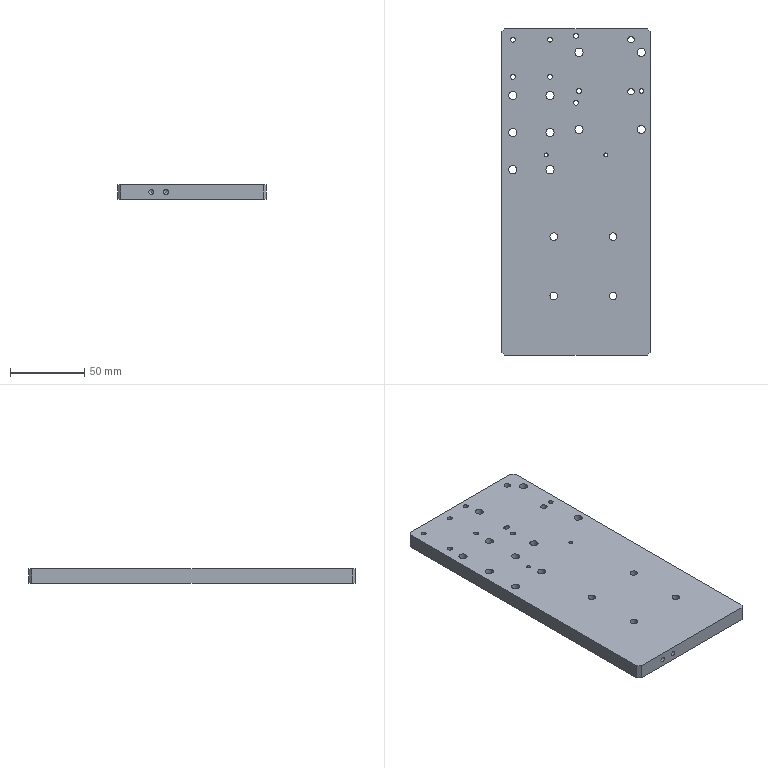CAM job | NX | 3-axis milling, drilling | part box 100 x 220 x 10 mm | stock box 105 x 225 x 12 mm
Tools:
number,name,description,diameter,corner_radius,flute_length,length,flutes
19,D2,平底铣刀-粗,2.0,0.0,50.0,75.0,2
4,D4,平底铣刀-粗,4.0,0.0,25.0,75.0,2
6,D6,平底铣刀-粗,6.0,0.0,25.0,75.0,2
9,D10,平底铣刀-粗,10.0,0.0,35.0,75.0,2
23,D2-J,平底铣刀-精,2.0,0.0,50.0,75.0,2
11,D4-J,平底铣刀-精,4.0,0.0,50.0,75.0,2
7,D6-J,平底铣刀-精,6.0,0.0,25.0,75.0,2
10,D10-J,平底铣刀-精,10.0,0.0,35.0,75.0,2
1,D80R0.8飞刀,圆鼻刀-粗,80.0,0.8,50.0,75.0,2
1,D80R0.8飞刀-J,圆鼻刀-精,80.0,0.8,50.0,75.0,2
2,D6倒角刀,倒角刀,6.0,0.0,3.0,25.0,2
20,M3X0.5,丝锥,2.5,0.0,35.0,50.0,2
21,M4X0.7,丝锥,3.3,0.0,35.0,50.0,2
22,M5X0.8,丝锥,4.2,0.0,35.0,50.0,2
16,M6X1.0,丝锥,5.0,0.0,35.0,50.0,2
24,D3铰刀,Drilling Tool,3.0,0.0,75.0,100.0,6
12,ZT2.5,钻头,2.5,0.0,35.0,50.0,2
15,ZT5,钻头,5.0,0.0,35.0,50.0,2
18,ZT5.5,钻头,5.5,0.0,35.0,50.0,2
13,钻头3.3,Twist Drill 3.3 mm,3.3,0.0,35.0,35.008,2
14,钻头4.2,Twist Drill 4.2 mm,4.2,0.0,41.0,41.738,2
17,ZT2.9,Drilling Tool,2.9,0.0,35.0,50.0,2
Operations:
program,operation,operation_type,tool,method,geometry_group,spindle_rpm,surface_speed,feed_per_tooth,feed_cut,feed_plunge,cut_length_mm,path_length_mm,cut_time_min,machine_time_min
B,底壁铣飞面开粗_COPY,VolumeBased25DMillingOperation,D80R0.8飞刀,分层开粗-切深K-步距G,W-B,2800.0,703.696,0.5357,3000.0,100.0,2666.79,2835.673,0.8889,0.9058
B,底壁铣飞面精光_COPY,VolumeBased25DMillingOperation,D80R0.8飞刀-J,侧刃精光-切深K-步距G,W-B,4000.0,1005.28,0.125,1000.0,100.0,666.11,702.11,0.6661,0.6697
B,钻倒角_4,Operation,D6倒角刀,METHOD,W-B,8000.0,150.796,0.0625,1000.0,0.0,9.5,102.112,0.0095,0.0188
B,钻倒角_5,Operation,D6倒角刀,METHOD,W-B,8000.0,150.796,0.0625,1000.0,0.0,4.8,49.6,0.0048,0.0093
B,钻倒角_6,Operation,D6倒角刀,METHOD,W-B,8000.0,150.796,0.0625,1000.0,0.0,31.2,235.798,0.0312,0.0517
B,钻倒角_7,Operation,D6倒角刀,METHOD,W-B,8000.0,150.796,0.0625,1000.0,0.0,11.4,100.928,0.0114,0.0204
B,铣倒角_5,PlanarMilling,D6倒角刀,METHOD,W-B,8000.0,150.796,0.0375,600.0,100.0,75.821,364.836,0.1264,0.1553
B,铣倒角_6,PlanarMilling,D6倒角刀,METHOD,W-B,8000.0,150.796,0.075,1200.0,100.0,177.946,861.886,0.1483,0.2167
B,C0.3封闭铣廓倒角6X45L_COPY,PlanarMilling,D6倒角刀,爬面_倒角-切深0-步距G,W-B,7000.0,131.0,0.1071,1500.0,100.0,673.102,930.341,0.4487,0.4745
A,顶面,FaceMilling,D80R0.8飞刀,侧刃精光-切深K-步距G,W-A,4000.0,1005.31,0.125,1000.0,100.0,1004.0,1040.0,1.004,1.008
A,外形粗_2,VolumeBased25DMillingOperation,D10,METHOD,W-A,8000.0,251.327,0.3125,5000.0,80.0,10011.875,10060.475,2.002,2.007
A,打点-深0.8,Operation,D6倒角刀,NONE,W-A,8000.0,150.796,0.0312,500.0,90.0,50.4,871.238,0.1008,0.1829
A,通孔-M3螺纹底孔,Operation,ZT2.5,NONE,W-A,3000.0,23.562,0.05,300.0,90.0,33.502,148.017,0.1117,0.1231
A,通孔-精孔3.0预钻,Operation,ZT2.9,NONE,W-A,3200.0,29.154,0.0312,200.0,90.0,29.674,141.861,0.1484,0.1596
A,通孔-M4螺纹底孔,Operation,钻头3.3,NONE,W-A,3000.0,31.102,0.05,300.0,90.0,101.948,366.432,0.3398,0.3663
A,通孔-M5螺纹底孔,Operation,钻头4.2,NONE,W-A,3000.0,39.584,0.0583,350.0,90.0,36.524,149.061,0.1044,0.1156
A,通孔-M6螺纹底孔,Operation,ZT5,NONE,W-A,2800.0,43.982,0.0625,350.0,90.0,74.009,311.055,0.2115,0.2352
A,沉头孔-钻孔0段,Operation,ZT5.5,NONE,W-A,1200.0,20.735,0.0625,150.0,90.0,146.524,605.76,0.9768,1.023
A,通孔-精孔6.0预钻14.8,Operation,ZT5.5,NONE,W-A,2500.0,45.553,0.03,150.0,90.0,19.405,119.823,0.1294,0.1394
A,通腰槽粗_1,VolumeBased25DMillingOperation,D2,METHOD,W-A,6000.0,37.699,0.0417,500.0,100.0,522.974,571.674,1.046,1.051
A,铣孔开粗D6_1,CylinderMilling,D6,NONE,W-A,8000.0,150.796,0.075,1200.0,100.0,1588.996,2301.545,1.324,1.395
A,铣孔开粗D4_1,CylinderMilling,D4,NONE,W-A,8000.0,100.531,0.0375,600.0,100.0,313.409,446.409,0.5223,0.5356
A,铣孔精光D6_1,CylinderMilling,D6-J,精光步距切深关,W-A,8000.0,150.796,0.0312,500.0,100.0,333.986,1051.534,0.668,0.7397
A,仅选体,SurfaceContour,D6倒角刀,METHOD,W-A,8000.0,150.796,0.1875,3000.0,100.0,665.713,820.009,0.2219,0.2373
A,钻倒角_1,Operation,D6倒角刀,METHOD,W-A,8000.0,150.796,0.0312,500.0,0.0,9.5,102.112,0.019,0.0283
A,钻倒角_2,Operation,D6倒角刀,METHOD,W-A,8000.0,150.796,0.0312,500.0,0.0,4.8,49.6,0.0096,0.0141
A,钻倒角_3,Operation,D6倒角刀,METHOD,W-A,8000.0,150.796,0.0312,500.0,0.0,31.2,235.798,0.0624,0.0829
A,铣倒角_1,PlanarMilling,D6倒角刀,METHOD,W-A,8000.0,150.796,0.0312,500.0,100.0,36.041,154.428,0.0721,0.0839
A,铣倒角_2,PlanarMilling,D6倒角刀,METHOD,W-A,8000.0,150.796,0.0312,500.0,100.0,79.753,364.605,0.1595,0.188
A,铣倒角_3,PlanarMilling,D6倒角刀,METHOD,W-A,8000.0,150.796,0.0312,500.0,100.0,41.927,161.633,0.0839,0.0958
A,铣倒角_4,PlanarMilling,D6倒角刀,NONE,W-A,8000.0,150.796,0.05,800.0,100.0,402.51,1022.014,0.5031,0.5651
A,铣孔精光D4-J_1,CylinderMilling,D4-J,精光步距切深关,W-A,8000.0,100.531,0.0125,200.0,100.0,115.195,248.195,0.576,0.5893
A,腰槽精_1,VolumeBased25DMillingOperation,D2-J,METHOD,W-A,6000.0,113.0,0.0167,200.0,100.0,45.035,125.95,0.2252,0.2333
A,铰孔,Operation,D3铰刀,METHOD,W-A,500.0,4.712,0.0167,50.0,0.0,12.0,64.0,0.24,0.2452
A,通孔-攻牙M3,Operation,M3X0.5,METHOD,W-A,800.0,6.283,0.0003,0.5,90.0,28.0,137.012,56.0,56.011
A,通孔-攻牙M4,Operation,M4X0.7,METHOD,W-A,600.0,6.22,0.0006,0.7,90.0,84.0,330.535,120.0,120.025
A,通孔-攻牙M5,Operation,M5X0.8,METHOD,W-A,500.0,6.597,0.0008,0.8,90.0,29.0,134.014,36.25,36.261
A,通孔-攻牙M6,Operation,M6X1.0,METHOD,W-A,500.0,7.854,0.001,1.0,90.0,58.0,279.038,58.0,58.022
A,外形半精_2,VolumeBased25DMillingOperation,D10-J,METHOD,W-A,8000.0,251.327,0.0625,1000.0,100.0,671.688,730.888,0.6717,0.6776